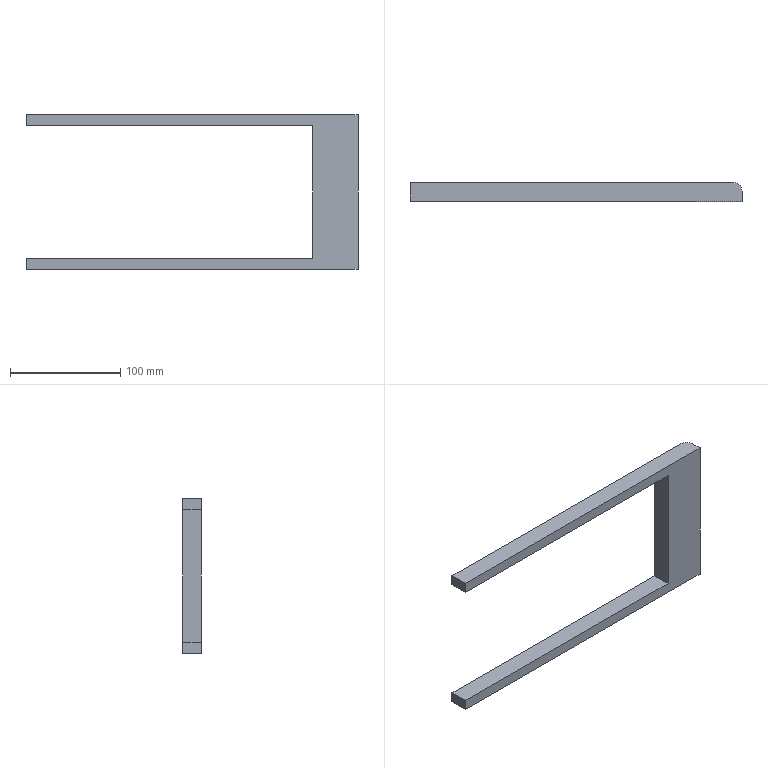Part | Creo | features CURVE 3, DATUM PLANE 3, PROTRUSION 2, COORDINATE SYSTEM 1, CUT 1, ROUND 1 | 1 solid | 11 faces | volume 184057 mm3 | plane 10 | cylinder 1 | commonest cylinder face diameters 16 x1